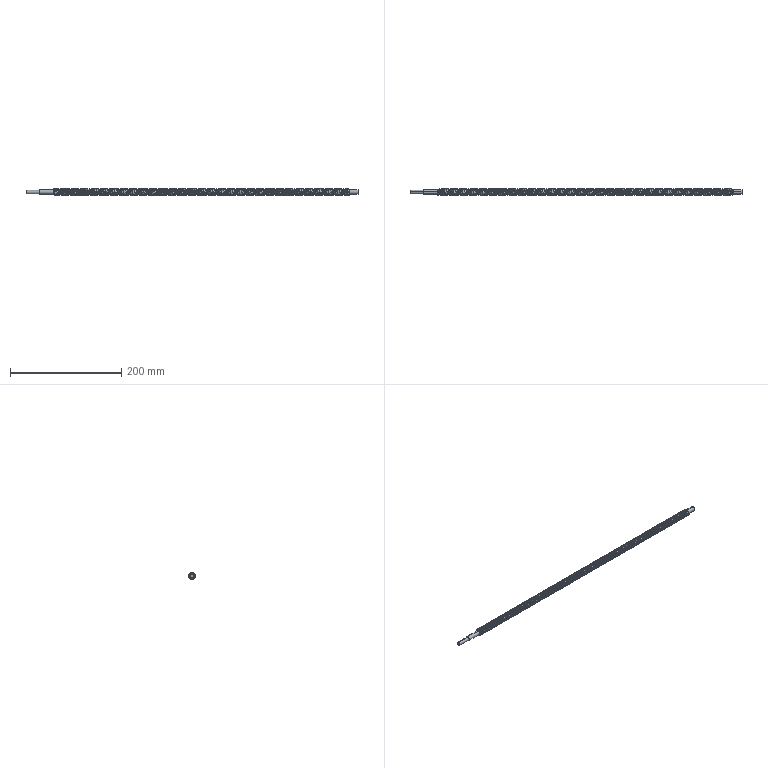Part | SolidWorks | features BaseBody 1 | 1 solid | 345 faces | box 596 x 12 x 12 mm | volume 49548 mm3 | cylinder 273 | spline 67 | plane 5 | commonest cylinder face diameters 12 x267 8 x4 6 x2